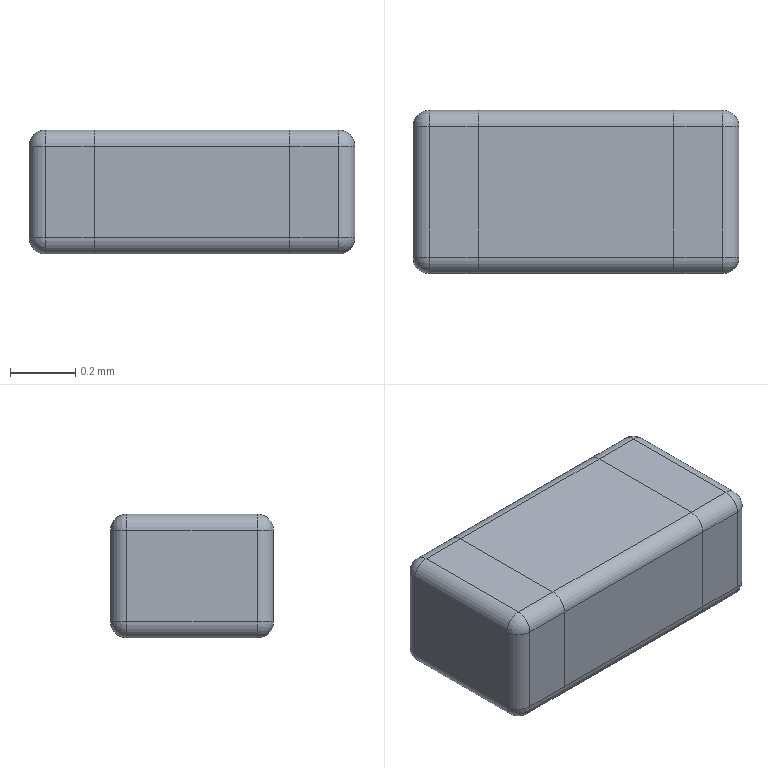Part | STEP file | RJ-USIO-V1_2-220411_10 | 1 solid | 42 faces | box 1 x 0.5 x 0.38 mm | volume 0.1861 mm3 | cylinder 20 | plane 14 | sphere 8 | commonest cylinder face diameters 0.1 x20